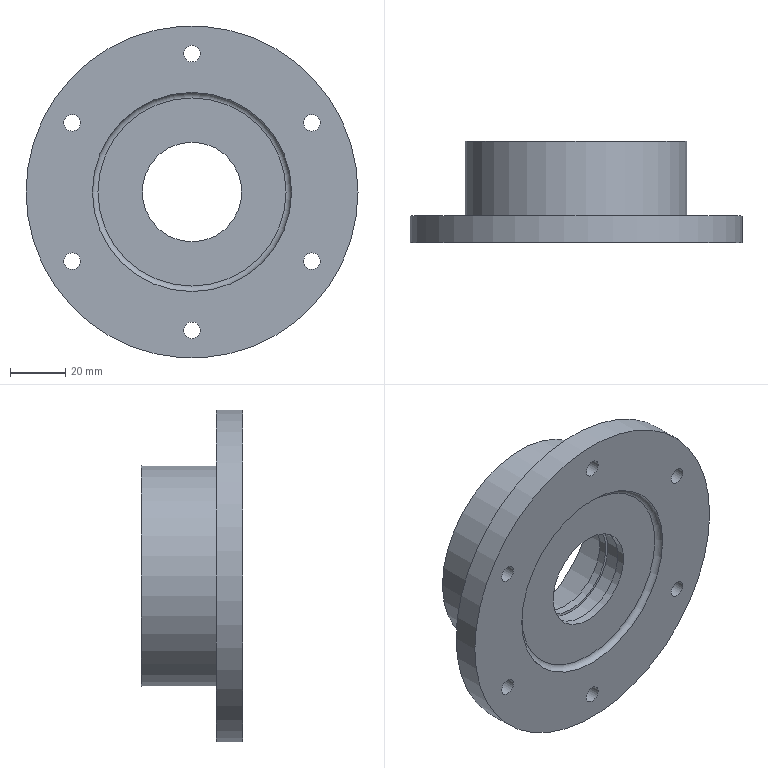Part | NX | features DATUM_CSYS 10, HOLE PACKAGE 9, SIMPLE HOLE 9, SKETCH 9, EXTRACT_DATUM_AXIS 6, EXTRACT_FACE 6, Instance Feature 5, BLEND 2, EXTRUDE 2, Pattern Feature 1, SWP104 1 | 1 solid | 21 faces | box 120 x 36.6 x 120 mm | volume 131277 mm3 | cylinder 12 | plane 5 | torus 2 | cone 2 | commonest cylinder face diameters 6 x6 36 x2 37.948 x1 72 x1 80 x1 120 x1
STEP:
#1=CARTESIAN_POINT('',(0.,-4.657,18.));
#2=VERTEX_POINT('',#1);
#3=CARTESIAN_POINT('',(0.,-4.657,0.));
#4=DIRECTION('',(0.,1.,0.));
#5=DIRECTION('',(0.,0.,1.));
#6=AXIS2_PLACEMENT_3D('',#3,#4,#5);
#7=CIRCLE('',#6,18.);
#8=EDGE_CURVE('',#2,#2,#7,.T.);
#9=ORIENTED_EDGE('',*,*,#8,.T.);
#10=EDGE_LOOP('',(#9));
#11=FACE_BOUND('',#10,.T.);
#12=CARTESIAN_POINT('',(0.,-7.6,18.));
#13=VERTEX_POINT('',#12);
#14=CARTESIAN_POINT('',(0.,-7.6,0.));
#15=DIRECTION('',(0.,1.,0.));
#16=DIRECTION('',(0.,0.,1.));
#17=AXIS2_PLACEMENT_3D('',#14,#15,#16);
#18=CIRCLE('',#17,18.);
#19=EDGE_CURVE('',#13,#13,#18,.F.);
#20=ORIENTED_EDGE('',*,*,#19,.T.);
#21=EDGE_LOOP('',(#20));
#22=FACE_BOUND('',#21,.T.);
#23=CARTESIAN_POINT('',(0.,27.,0.));
#24=DIRECTION('',(0.,-1.,0.));
#25=DIRECTION('',(0.,0.,-1.));
#26=AXIS2_PLACEMENT_3D('',#23,#24,#25);
#27=CYLINDRICAL_SURFACE('',#26,18.);
#28=ADVANCED_FACE('',(#11,#22),#27,.F.);
#29=CARTESIAN_POINT('',(60.,0.,0.));
#30=VERTEX_POINT('',#29);
#31=CARTESIAN_POINT('',(0.,0.,0.));
#32=DIRECTION('',(0.,-1.,0.));
#33=DIRECTION('',(1.,0.,0.));
#34=AXIS2_PLACEMENT_3D('',#31,#32,#33);
#35=CIRCLE('',#34,60.);
#36=EDGE_CURVE('',#30,#30,#35,.T.);
#37=ORIENTED_EDGE('',*,*,#36,.T.);
#38=EDGE_LOOP('',(#37));
#39=FACE_BOUND('',#38,.T.);
#40=CARTESIAN_POINT('',(60.,-9.6,0.));
#41=VERTEX_POINT('',#40);
#42=CARTESIAN_POINT('',(0.,-9.6,0.));
#43=DIRECTION('',(0.,-1.,0.));
#44=DIRECTION('',(1.,0.,0.));
#45=AXIS2_PLACEMENT_3D('',#42,#43,#44);
#46=CIRCLE('',#45,60.);
#47=EDGE_CURVE('',#41,#41,#46,.T.);
#48=ORIENTED_EDGE('',*,*,#47,.F.);
#49=EDGE_LOOP('',(#48));
#50=FACE_BOUND('',#49,.T.);
#51=CARTESIAN_POINT('',(0.,0.,0.));
#52=DIRECTION('',(0.,-1.,0.));
#53=DIRECTION('',(0.,0.,-1.));
#54=AXIS2_PLACEMENT_3D('',#51,#52,#53);
#55=CYLINDRICAL_SURFACE('',#54,60.);
#56=ADVANCED_FACE('',(#39,#50),#55,.T.);
#57=CARTESIAN_POINT('',(-43.301,0.,22.));
#58=VERTEX_POINT('',#57);
#59=CARTESIAN_POINT('',(-43.301,0.,25.));
#60=DIRECTION('',(0.,-1.,0.));
#61=DIRECTION('',(0.,0.,-1.));
#62=AXIS2_PLACEMENT_3D('',#59,#60,#61);
#63=CIRCLE('',#62,3.);
#64=EDGE_CURVE('',#58,#58,#63,.T.);
#65=ORIENTED_EDGE('',*,*,#64,.T.);
#66=EDGE_LOOP('',(#65));
#67=FACE_BOUND('',#66,.T.);
#68=CARTESIAN_POINT('',(-43.301,0.,-28.));
#69=VERTEX_POINT('',#68);
#70=CARTESIAN_POINT('',(-43.301,0.,-25.));
#71=DIRECTION('',(0.,-1.,0.));
#72=DIRECTION('',(0.,0.,-1.));
#73=AXIS2_PLACEMENT_3D('',#70,#71,#72);
#74=CIRCLE('',#73,3.);
#75=EDGE_CURVE('',#69,#69,#74,.T.);
#76=ORIENTED_EDGE('',*,*,#75,.T.);
#77=EDGE_LOOP('',(#76));
#78=FACE_BOUND('',#77,.T.);
#79=CARTESIAN_POINT('',(0.,0.,-53.));
#80=VERTEX_POINT('',#79);
#81=CARTESIAN_POINT('',(0.,0.,-50.));
#82=DIRECTION('',(0.,-1.,0.));
#83=DIRECTION('',(0.,0.,-1.));
#84=AXIS2_PLACEMENT_3D('',#81,#82,#83);
#85=CIRCLE('',#84,3.);
#86=EDGE_CURVE('',#80,#80,#85,.T.);
#87=ORIENTED_EDGE('',*,*,#86,.T.);
#88=EDGE_LOOP('',(#87));
#89=FACE_BOUND('',#88,.T.);
#90=CARTESIAN_POINT('',(43.301,0.,-28.));
#91=VERTEX_POINT('',#90);
#92=CARTESIAN_POINT('',(43.301,0.,-25.));
#93=DIRECTION('',(0.,-1.,0.));
#94=DIRECTION('',(0.,0.,-1.));
#95=AXIS2_PLACEMENT_3D('',#92,#93,#94);
#96=CIRCLE('',#95,3.);
#97=EDGE_CURVE('',#91,#91,#96,.T.);
#98=ORIENTED_EDGE('',*,*,#97,.T.);
#99=EDGE_LOOP('',(#98));
#100=FACE_BOUND('',#99,.T.);
#101=CARTESIAN_POINT('',(43.301,0.,22.));
#102=VERTEX_POINT('',#101);
#103=CARTESIAN_POINT('',(43.301,0.,25.));
#104=DIRECTION('',(0.,-1.,0.));
#105=DIRECTION('',(0.,0.,-1.));
#106=AXIS2_PLACEMENT_3D('',#103,#104,#105);
#107=CIRCLE('',#106,3.);
#108=EDGE_CURVE('',#102,#102,#107,.T.);
#109=ORIENTED_EDGE('',*,*,#108,.T.);
#110=EDGE_LOOP('',(#109));
#111=FACE_BOUND('',#110,.T.);
#112=CARTESIAN_POINT('',(0.,0.,47.));
#113=VERTEX_POINT('',#112);
#114=CARTESIAN_POINT('',(0.,0.,50.));
#115=DIRECTION('',(0.,-1.,0.));
#116=DIRECTION('',(0.,0.,-1.));
#117=AXIS2_PLACEMENT_3D('',#114,#115,#116);
#118=CIRCLE('',#117,3.);
#119=EDGE_CURVE('',#113,#113,#118,.T.);
#120=ORIENTED_EDGE('',*,*,#119,.T.);
#121=EDGE_LOOP('',(#120));
#122=FACE_BOUND('',#121,.T.);
#123=CARTESIAN_POINT('',(40.,0.,0.));
#124=VERTEX_POINT('',#123);
#125=CARTESIAN_POINT('',(0.,0.,0.));
#126=DIRECTION('',(0.,1.,0.));
#127=DIRECTION('',(1.,0.,0.));
#128=AXIS2_PLACEMENT_3D('',#125,#126,#127);
#129=CIRCLE('',#128,40.);
#130=EDGE_CURVE('',#124,#124,#129,.T.);
#131=ORIENTED_EDGE('',*,*,#130,.F.);
#132=EDGE_LOOP('',(#131));
#133=FACE_BOUND('',#132,.T.);
#134=ORIENTED_EDGE('',*,*,#36,.F.);
#135=EDGE_LOOP('',(#134));
#136=FACE_BOUND('',#135,.T.);
#137=CARTESIAN_POINT('',(0.,0.,0.));
#138=DIRECTION('',(0.,-1.,0.));
#139=DIRECTION('',(0.,0.,-1.));
#140=AXIS2_PLACEMENT_3D('',#137,#138,#139);
#141=PLANE('',#140);
#142=ADVANCED_FACE('',(#67,#78,#89,#100,#111,#122,#133,#136),#141,.F.);
#143=CARTESIAN_POINT('',(-43.301,-9.6,28.));
#144=VERTEX_POINT('',#143);
#145=CARTESIAN_POINT('',(-43.301,-9.6,25.));
#146=DIRECTION('',(0.,1.,0.));
#147=DIRECTION('',(0.,0.,1.));
#148=AXIS2_PLACEMENT_3D('',#145,#146,#147);
#149=CIRCLE('',#148,3.);
#150=EDGE_CURVE('',#144,#144,#149,.T.);
#151=ORIENTED_EDGE('',*,*,#150,.T.);
#152=EDGE_LOOP('',(#151));
#153=FACE_BOUND('',#152,.T.);
#154=CARTESIAN_POINT('',(-43.301,-9.6,-22.));
#155=VERTEX_POINT('',#154);
#156=CARTESIAN_POINT('',(-43.301,-9.6,-25.));
#157=DIRECTION('',(0.,1.,0.));
#158=DIRECTION('',(0.,0.,1.));
#159=AXIS2_PLACEMENT_3D('',#156,#157,#158);
#160=CIRCLE('',#159,3.);
#161=EDGE_CURVE('',#155,#155,#160,.T.);
#162=ORIENTED_EDGE('',*,*,#161,.T.);
#163=EDGE_LOOP('',(#162));
#164=FACE_BOUND('',#163,.T.);
#165=CARTESIAN_POINT('',(0.,-9.6,-47.));
#166=VERTEX_POINT('',#165);
#167=CARTESIAN_POINT('',(0.,-9.6,-50.));
#168=DIRECTION('',(0.,1.,0.));
#169=DIRECTION('',(0.,0.,1.));
#170=AXIS2_PLACEMENT_3D('',#167,#168,#169);
#171=CIRCLE('',#170,3.);
#172=EDGE_CURVE('',#166,#166,#171,.T.);
#173=ORIENTED_EDGE('',*,*,#172,.T.);
#174=EDGE_LOOP('',(#173));
#175=FACE_BOUND('',#174,.T.);
#176=CARTESIAN_POINT('',(43.301,-9.6,-22.));
#177=VERTEX_POINT('',#176);
#178=CARTESIAN_POINT('',(43.301,-9.6,-25.));
#179=DIRECTION('',(0.,1.,0.));
#180=DIRECTION('',(0.,0.,1.));
#181=AXIS2_PLACEMENT_3D('',#178,#179,#180);
#182=CIRCLE('',#181,3.);
#183=EDGE_CURVE('',#177,#177,#182,.T.);
#184=ORIENTED_EDGE('',*,*,#183,.T.);
#185=EDGE_LOOP('',(#184));
#186=FACE_BOUND('',#185,.T.);
#187=CARTESIAN_POINT('',(43.301,-9.6,28.));
#188=VERTEX_POINT('',#187);
#189=CARTESIAN_POINT('',(43.301,-9.6,25.));
#190=DIRECTION('',(0.,1.,0.));
#191=DIRECTION('',(0.,0.,1.));
#192=AXIS2_PLACEMENT_3D('',#189,#190,#191);
#193=CIRCLE('',#192,3.);
#194=EDGE_CURVE('',#188,#188,#193,.T.);
#195=ORIENTED_EDGE('',*,*,#194,.T.);
#196=EDGE_LOOP('',(#195));
#197=FACE_BOUND('',#196,.T.);
#198=CARTESIAN_POINT('',(0.,-9.6,53.));
#199=VERTEX_POINT('',#198);
#200=CARTESIAN_POINT('',(0.,-9.6,50.));
#201=DIRECTION('',(0.,1.,0.));
#202=DIRECTION('',(0.,0.,1.));
#203=AXIS2_PLACEMENT_3D('',#200,#201,#202);
#204=CIRCLE('',#203,3.);
#205=EDGE_CURVE('',#199,#199,#204,.T.);
#206=ORIENTED_EDGE('',*,*,#205,.T.);
#207=EDGE_LOOP('',(#206));
#208=FACE_BOUND('',#207,.T.);
#209=CARTESIAN_POINT('',(0.,-9.6,36.));
#210=VERTEX_POINT('',#209);
#211=CARTESIAN_POINT('',(0.,-9.6,0.));
#212=DIRECTION('',(0.,1.,0.));
#213=DIRECTION('',(0.,0.,1.));
#214=AXIS2_PLACEMENT_3D('',#211,#212,#213);
#215=CIRCLE('',#214,36.);
#216=EDGE_CURVE('',#210,#210,#215,.T.);
#217=ORIENTED_EDGE('',*,*,#216,.T.);
#218=EDGE_LOOP('',(#217));
#219=FACE_BOUND('',#218,.T.);
#220=ORIENTED_EDGE('',*,*,#47,.T.);
#221=EDGE_LOOP('',(#220));
#222=FACE_BOUND('',#221,.T.);
#223=CARTESIAN_POINT('',(0.,-9.6,0.));
#224=DIRECTION('',(0.,-1.,0.));
#225=DIRECTION('',(0.,0.,-1.));
#226=AXIS2_PLACEMENT_3D('',#223,#224,#225);
#227=PLANE('',#226);
#228=ADVANCED_FACE('',(#153,#164,#175,#186,#197,#208,#219,#222),#227,.T.);
#229=ORIENTED_EDGE('',*,*,#130,.T.);
#230=EDGE_LOOP('',(#229));
#231=FACE_BOUND('',#230,.T.);
#232=CARTESIAN_POINT('',(40.,27.,0.));
#233=VERTEX_POINT('',#232);
#234=CARTESIAN_POINT('',(0.,27.,0.));
#235=DIRECTION('',(0.,1.,0.));
#236=DIRECTION('',(1.,0.,0.));
#237=AXIS2_PLACEMENT_3D('',#234,#235,#236);
#238=CIRCLE('',#237,40.);
#239=EDGE_CURVE('',#233,#233,#238,.T.);
#240=ORIENTED_EDGE('',*,*,#239,.F.);
#241=EDGE_LOOP('',(#240));
#242=FACE_BOUND('',#241,.T.);
#243=CARTESIAN_POINT('',(0.,0.,0.));
#244=DIRECTION('',(0.,1.,0.));
#245=DIRECTION('',(0.,0.,1.));
#246=AXIS2_PLACEMENT_3D('',#243,#244,#245);
#247=CYLINDRICAL_SURFACE('',#246,40.);
#248=ADVANCED_FACE('',(#231,#242),#247,.T.);
#249=CARTESIAN_POINT('',(0.,27.,-36.));
#250=VERTEX_POINT('',#249);
#251=CARTESIAN_POINT('',(0.,27.,0.));
#252=DIRECTION('',(0.,-1.,0.));
#253=DIRECTION('',(0.,0.,-1.));
#254=AXIS2_PLACEMENT_3D('',#251,#252,#253);
#255=CIRCLE('',#254,36.);
#256=EDGE_CURVE('',#250,#250,#255,.T.);
#257=ORIENTED_EDGE('',*,*,#256,.T.);
#258=EDGE_LOOP('',(#257));
#259=FACE_BOUND('',#258,.T.);
#260=ORIENTED_EDGE('',*,*,#239,.T.);
#261=EDGE_LOOP('',(#260));
#262=FACE_BOUND('',#261,.T.);
#263=CARTESIAN_POINT('',(0.,27.,0.));
#264=DIRECTION('',(0.,1.,0.));
#265=DIRECTION('',(0.,0.,1.));
#266=AXIS2_PLACEMENT_3D('',#263,#264,#265);
#267=PLANE('',#266);
#268=ADVANCED_FACE('',(#259,#262),#267,.T.);
#269=CARTESIAN_POINT('',(0.,4.5,-31.));
#270=VERTEX_POINT('',#269);
#271=CARTESIAN_POINT('',(0.,4.5,0.));
#272=DIRECTION('',(0.,-1.,0.));
#273=DIRECTION('',(0.,0.,-1.));
#274=AXIS2_PLACEMENT_3D('',#271,#272,#273);
#275=CIRCLE('',#274,31.);
#276=EDGE_CURVE('',#270,#270,#275,.F.);
#277=ORIENTED_EDGE('',*,*,#276,.T.);
#278=EDGE_LOOP('',(#277));
#279=FACE_BOUND('',#278,.T.);
#280=CARTESIAN_POINT('',(0.,4.5,-18.));
#281=VERTEX_POINT('',#280);
#282=CARTESIAN_POINT('',(0.,4.5,0.));
#283=DIRECTION('',(0.,-1.,0.));
#284=DIRECTION('',(0.,0.,-1.));
#285=AXIS2_PLACEMENT_3D('',#282,#283,#284);
#286=CIRCLE('',#285,18.);
#287=EDGE_CURVE('',#281,#281,#286,.T.);
#288=ORIENTED_EDGE('',*,*,#287,.T.);
#289=EDGE_LOOP('',(#288));
#290=FACE_BOUND('',#289,.T.);
#291=CARTESIAN_POINT('',(0.,4.5,0.));
#292=DIRECTION('',(0.,-1.,0.));
#293=DIRECTION('',(0.,0.,-1.));
#294=AXIS2_PLACEMENT_3D('',#291,#292,#293);
#295=PLANE('',#294);
#296=ADVANCED_FACE('',(#279,#290),#295,.F.);
#297=CARTESIAN_POINT('',(0.,9.5,-36.));
#298=VERTEX_POINT('',#297);
#299=CARTESIAN_POINT('',(0.,9.5,0.));
#300=DIRECTION('',(0.,-1.,0.));
#301=DIRECTION('',(0.,0.,-1.));
#302=AXIS2_PLACEMENT_3D('',#299,#300,#301);
#303=CIRCLE('',#302,36.);
#304=EDGE_CURVE('',#298,#298,#303,.T.);
#305=ORIENTED_EDGE('',*,*,#304,.T.);
#306=EDGE_LOOP('',(#305));
#307=FACE_BOUND('',#306,.T.);
#308=ORIENTED_EDGE('',*,*,#256,.F.);
#309=EDGE_LOOP('',(#308));
#310=FACE_BOUND('',#309,.T.);
#311=CARTESIAN_POINT('',(0.,27.,0.));
#312=DIRECTION('',(0.,-1.,0.));
#313=DIRECTION('',(0.,0.,-1.));
#314=AXIS2_PLACEMENT_3D('',#311,#312,#313);
#315=CYLINDRICAL_SURFACE('',#314,36.);
#316=ADVANCED_FACE('',(#307,#310),#315,.F.);
#317=CARTESIAN_POINT('',(0.,1.445,-18.));
#318=VERTEX_POINT('',#317);
#319=CARTESIAN_POINT('',(0.,1.445,0.));
#320=DIRECTION('',(0.,-1.,0.));
#321=DIRECTION('',(0.,0.,-1.));
#322=AXIS2_PLACEMENT_3D('',#319,#320,#321);
#323=CIRCLE('',#322,18.);
#324=EDGE_CURVE('',#318,#318,#323,.T.);
#325=ORIENTED_EDGE('',*,*,#324,.T.);
#326=EDGE_LOOP('',(#325));
#327=FACE_BOUND('',#326,.T.);
#328=ORIENTED_EDGE('',*,*,#287,.F.);
#329=EDGE_LOOP('',(#328));
#330=FACE_BOUND('',#329,.T.);
#331=CARTESIAN_POINT('',(0.,27.,0.));
#332=DIRECTION('',(0.,-1.,0.));
#333=DIRECTION('',(0.,0.,-1.));
#334=AXIS2_PLACEMENT_3D('',#331,#332,#333);
#335=CYLINDRICAL_SURFACE('',#334,18.);
#336=ADVANCED_FACE('',(#327,#330),#335,.F.);
#337=CARTESIAN_POINT('',(0.,-7.6,34.));
#338=VERTEX_POINT('',#337);
#339=CARTESIAN_POINT('',(0.,-7.6,0.));
#340=DIRECTION('',(0.,1.,0.));
#341=DIRECTION('',(0.,0.,1.));
#342=AXIS2_PLACEMENT_3D('',#339,#340,#341);
#343=CIRCLE('',#342,34.);
#344=EDGE_CURVE('',#338,#338,#343,.F.);
#345=ORIENTED_EDGE('',*,*,#344,.T.);
#346=EDGE_LOOP('',(#345));
#347=FACE_BOUND('',#346,.T.);
#348=ORIENTED_EDGE('',*,*,#19,.F.);
#349=EDGE_LOOP('',(#348));
#350=FACE_BOUND('',#349,.T.);
#351=CARTESIAN_POINT('',(0.,-7.6,0.));
#352=DIRECTION('',(0.,1.,0.));
#353=DIRECTION('',(0.,0.,1.));
#354=AXIS2_PLACEMENT_3D('',#351,#352,#353);
#355=PLANE('',#354);
#356=ADVANCED_FACE('',(#347,#350),#355,.F.);
#357=ORIENTED_EDGE('',*,*,#216,.F.);
#358=EDGE_LOOP('',(#357));
#359=FACE_BOUND('',#358,.T.);
#360=ORIENTED_EDGE('',*,*,#344,.F.);
#361=EDGE_LOOP('',(#360));
#362=FACE_BOUND('',#361,.T.);
#363=CARTESIAN_POINT('',(0.,-9.6,0.));
#364=DIRECTION('',(0.,1.,0.));
#365=DIRECTION('',(0.,0.,1.));
#366=AXIS2_PLACEMENT_3D('',#363,#364,#365);
#367=TOROIDAL_SURFACE('',#366,34.,2.);
#368=ADVANCED_FACE('',(#359,#362),#367,.F.);
#369=CARTESIAN_POINT('',(0.,-4.606,-18.974));
#370=VERTEX_POINT('',#369);
#371=CARTESIAN_POINT('',(0.,-4.606,0.));
#372=DIRECTION('',(0.,-1.,0.));
#373=DIRECTION('',(0.,0.,-1.));
#374=AXIS2_PLACEMENT_3D('',#371,#372,#373);
#375=CIRCLE('',#374,18.974);
#376=EDGE_CURVE('',#370,#370,#375,.F.);
#377=ORIENTED_EDGE('',*,*,#376,.T.);
#378=EDGE_LOOP('',(#377));
#379=FACE_BOUND('',#378,.T.);
#380=ORIENTED_EDGE('',*,*,#8,.F.);
#381=EDGE_LOOP('',(#380));
#382=FACE_BOUND('',#381,.T.);
#383=CARTESIAN_POINT('',(0.,-5.6,0.));
#384=DIRECTION('',(0.,1.,0.));
#385=DIRECTION('',(0.,0.,1.));
#386=AXIS2_PLACEMENT_3D('',#383,#384,#385);
#387=CONICAL_SURFACE('',#386,0.,1.518);
#388=ADVANCED_FACE('',(#379,#382),#387,.F.);
#389=CARTESIAN_POINT('',(0.,1.394,-18.974));
#390=VERTEX_POINT('',#389);
#391=CARTESIAN_POINT('',(0.,1.394,0.));
#392=DIRECTION('',(0.,-1.,0.));
#393=DIRECTION('',(0.,0.,-1.));
#394=AXIS2_PLACEMENT_3D('',#391,#392,#393);
#395=CIRCLE('',#394,18.974);
#396=EDGE_CURVE('',#390,#390,#395,.F.);
#397=ORIENTED_EDGE('',*,*,#396,.F.);
#398=EDGE_LOOP('',(#397));
#399=FACE_BOUND('',#398,.T.);
#400=ORIENTED_EDGE('',*,*,#324,.F.);
#401=EDGE_LOOP('',(#400));
#402=FACE_BOUND('',#401,.T.);
#403=CARTESIAN_POINT('',(0.,1.394,0.));
#404=DIRECTION('',(0.,-1.,0.));
#405=DIRECTION('',(0.,0.,-1.));
#406=AXIS2_PLACEMENT_3D('',#403,#404,#405);
#407=CONICAL_SURFACE('',#406,18.974,1.518);
#408=ADVANCED_FACE('',(#399,#402),#407,.F.);
#409=ORIENTED_EDGE('',*,*,#396,.T.);
#410=EDGE_LOOP('',(#409));
#411=FACE_BOUND('',#410,.T.);
#412=ORIENTED_EDGE('',*,*,#376,.F.);
#413=EDGE_LOOP('',(#412));
#414=FACE_BOUND('',#413,.T.);
#415=CARTESIAN_POINT('',(0.,-9.6,0.));
#416=DIRECTION('',(0.,-1.,0.));
#417=DIRECTION('',(0.,0.,-1.));
#418=AXIS2_PLACEMENT_3D('',#415,#416,#417);
#419=CYLINDRICAL_SURFACE('',#418,18.974);
#420=ADVANCED_FACE('',(#411,#414),#419,.F.);
#421=ORIENTED_EDGE('',*,*,#304,.F.);
#422=EDGE_LOOP('',(#421));
#423=FACE_BOUND('',#422,.T.);
#424=ORIENTED_EDGE('',*,*,#276,.F.);
#425=EDGE_LOOP('',(#424));
#426=FACE_BOUND('',#425,.T.);
#427=CARTESIAN_POINT('',(0.,9.5,0.));
#428=DIRECTION('',(0.,-1.,0.));
#429=DIRECTION('',(0.,0.,-1.));
#430=AXIS2_PLACEMENT_3D('',#427,#428,#429);
#431=TOROIDAL_SURFACE('',#430,31.,5.);
#432=ADVANCED_FACE('',(#423,#426),#431,.F.);
#433=ORIENTED_EDGE('',*,*,#205,.F.);
#434=EDGE_LOOP('',(#433));
#435=FACE_BOUND('',#434,.T.);
#436=ORIENTED_EDGE('',*,*,#119,.F.);
#437=EDGE_LOOP('',(#436));
#438=FACE_BOUND('',#437,.T.);
#439=CARTESIAN_POINT('',(0.,-9.6,50.));
#440=DIRECTION('',(0.,1.,0.));
#441=DIRECTION('',(0.,0.,1.));
#442=AXIS2_PLACEMENT_3D('',#439,#440,#441);
#443=CYLINDRICAL_SURFACE('',#442,3.);
#444=ADVANCED_FACE('',(#435,#438),#443,.F.);
#445=ORIENTED_EDGE('',*,*,#194,.F.);
#446=EDGE_LOOP('',(#445));
#447=FACE_BOUND('',#446,.T.);
#448=ORIENTED_EDGE('',*,*,#108,.F.);
#449=EDGE_LOOP('',(#448));
#450=FACE_BOUND('',#449,.T.);
#451=CARTESIAN_POINT('',(43.301,-9.6,25.));
#452=DIRECTION('',(0.,1.,0.));
#453=DIRECTION('',(0.,0.,1.));
#454=AXIS2_PLACEMENT_3D('',#451,#452,#453);
#455=CYLINDRICAL_SURFACE('',#454,3.);
#456=ADVANCED_FACE('',(#447,#450),#455,.F.);
#457=ORIENTED_EDGE('',*,*,#183,.F.);
#458=EDGE_LOOP('',(#457));
#459=FACE_BOUND('',#458,.T.);
#460=ORIENTED_EDGE('',*,*,#97,.F.);
#461=EDGE_LOOP('',(#460));
#462=FACE_BOUND('',#461,.T.);
#463=CARTESIAN_POINT('',(43.301,-9.6,-25.));
#464=DIRECTION('',(0.,1.,0.));
#465=DIRECTION('',(0.,0.,1.));
#466=AXIS2_PLACEMENT_3D('',#463,#464,#465);
#467=CYLINDRICAL_SURFACE('',#466,3.);
#468=ADVANCED_FACE('',(#459,#462),#467,.F.);
#469=ORIENTED_EDGE('',*,*,#172,.F.);
#470=EDGE_LOOP('',(#469));
#471=FACE_BOUND('',#470,.T.);
#472=ORIENTED_EDGE('',*,*,#86,.F.);
#473=EDGE_LOOP('',(#472));
#474=FACE_BOUND('',#473,.T.);
#475=CARTESIAN_POINT('',(0.,-9.6,-50.));
#476=DIRECTION('',(0.,1.,0.));
#477=DIRECTION('',(0.,0.,1.));
#478=AXIS2_PLACEMENT_3D('',#475,#476,#477);
#479=CYLINDRICAL_SURFACE('',#478,3.);
#480=ADVANCED_FACE('',(#471,#474),#479,.F.);
#481=ORIENTED_EDGE('',*,*,#161,.F.);
#482=EDGE_LOOP('',(#481));
#483=FACE_BOUND('',#482,.T.);
#484=ORIENTED_EDGE('',*,*,#75,.F.);
#485=EDGE_LOOP('',(#484));
#486=FACE_BOUND('',#485,.T.);
#487=CARTESIAN_POINT('',(-43.301,-9.6,-25.));
#488=DIRECTION('',(0.,1.,0.));
#489=DIRECTION('',(0.,0.,1.));
#490=AXIS2_PLACEMENT_3D('',#487,#488,#489);
#491=CYLINDRICAL_SURFACE('',#490,3.);
#492=ADVANCED_FACE('',(#483,#486),#491,.F.);
#493=ORIENTED_EDGE('',*,*,#150,.F.);
#494=EDGE_LOOP('',(#493));
#495=FACE_BOUND('',#494,.T.);
#496=ORIENTED_EDGE('',*,*,#64,.F.);
#497=EDGE_LOOP('',(#496));
#498=FACE_BOUND('',#497,.T.);
#499=CARTESIAN_POINT('',(-43.301,-9.6,25.));
#500=DIRECTION('',(0.,1.,0.));
#501=DIRECTION('',(0.,0.,1.));
#502=AXIS2_PLACEMENT_3D('',#499,#500,#501);
#503=CYLINDRICAL_SURFACE('',#502,3.);
#504=ADVANCED_FACE('',(#495,#498),#503,.F.);
#505=CLOSED_SHELL('',(#28,#56,#142,#228,#248,#268,#296,#316,#336,#356,#368,#388,#408,#420,#432,#444,#456,#468,#480,#492,#504));
#506=MANIFOLD_SOLID_BREP('',#505);
#507=(LENGTH_UNIT()NAMED_UNIT(*)SI_UNIT(.MILLI.,.METRE.));
#508=UNCERTAINTY_MEASURE_WITH_UNIT(LENGTH_MEASURE(0.00001),#507,'','');
#509=(NAMED_UNIT(*)PLANE_ANGLE_UNIT()SI_UNIT($,.RADIAN.));
#510=(NAMED_UNIT(*)SI_UNIT($,.STERADIAN.)SOLID_ANGLE_UNIT());
#511=(GEOMETRIC_REPRESENTATION_CONTEXT(3)GLOBAL_UNCERTAINTY_ASSIGNED_CONTEXT((#508))GLOBAL_UNIT_ASSIGNED_CONTEXT((#507,#509,#510))REPRESENTATION_CONTEXT('',''));
#512=ADVANCED_BREP_SHAPE_REPRESENTATION('',(#506),#511);